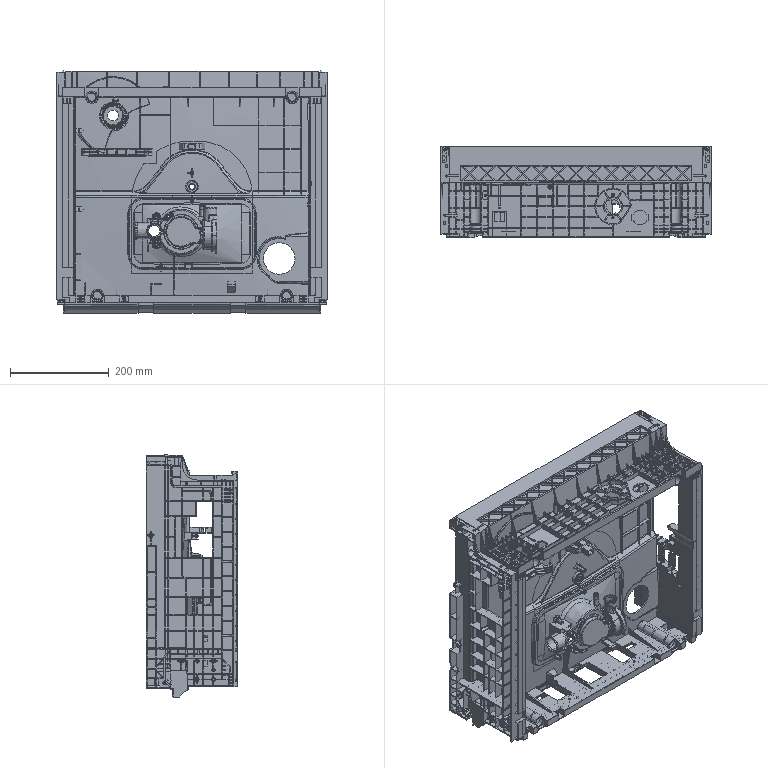Part | STEP file | DIZUO-XIN | 1 solid | 7386 faces | volume 2428763 mm3 | plane 4462 | cylinder 1436 | spline 754 | torus 353 | cone 260 | sphere 80 | other 41 | commonest cylinder face diameters 2 x279 1 x213 4 x125 0.6 x104 3.2 x83 6 x64